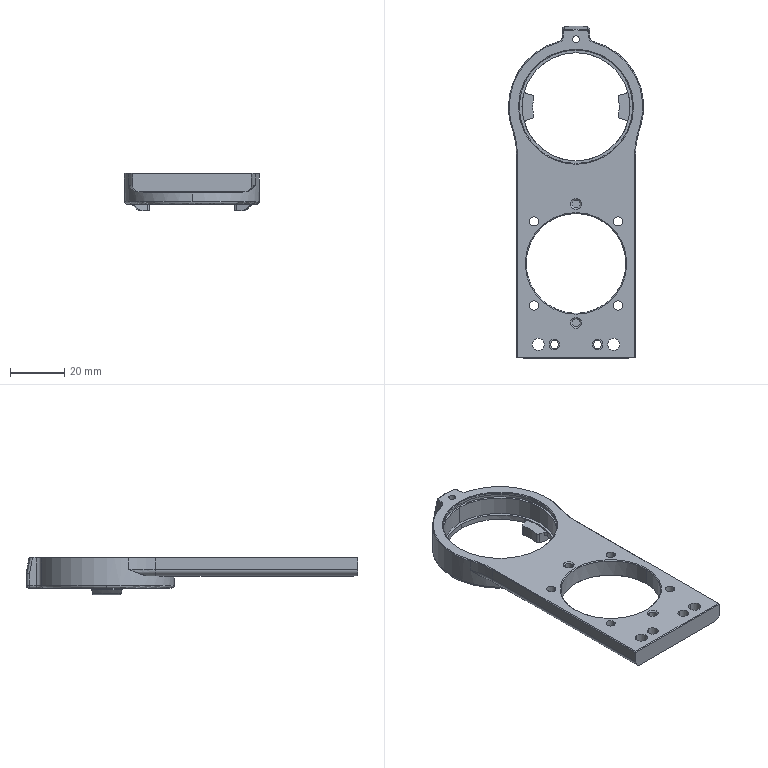NC program | NX | posted with a generic post | part box 50 x 122.9 x 14 mm
Lines 869 to 1773 of 10876:
(FLOOR_WALL_1_COPY_1 , TOOL : D4)
N1712 T11 M6
N1714 G54
N1716 G17 G0 G90 X62.415 Y-8.2 S9500 M3
N1718 G43 Z30. H11
N1720 Z-0.5
N1722 G94 G1 X62.153 Y-7.279 Z-0.55 F1000.
N1724 X61.62 Y-4.45 Z-0.701
N1726 X61.486 Y-3.078 Z-0.773
N1728 X61.34 Y-4.335 Z-0.84
N1730 X60.809 Y-6.819 Z-0.973
N1732 X60.044 Y-9.241 Z-1.106
N1734 X59.55 Y-10.406 Z-1.172
N1736 X59.81 Y-10.859 Z-1.2
N1738 X60.022 Y-11.336 Z-1.227
N1740 X63.435 Z-1.406
N1742 X62.941 Y-10.049 Z-1.478
N1744 X62.153 Y-7.279 Z-1.629
N1746 X61.62 Y-4.45 Z-1.78
N1748 X61.486 Y-3.078 Z-1.852
N1750 X61.34 Y-4.335 Z-1.918
N1752 X60.809 Y-6.819 Z-2.051
N1754 X60.044 Y-9.241 Z-2.185
N1756 X59.55 Y-10.406 Z-2.251
N1758 X59.81 Y-10.859 Z-2.278
N1760 X60.022 Y-11.336 Z-2.306
N1762 X61.728 Z-2.395
N1764 X63.435 F2000.
N1766 G2 X61.486 Y-3.078 R31.664
N1768 X59.55 Y-10.406 R26.664
N1770 X60.022 Y-11.336 R10.364
N1772 G1 X61.728
N1774 Y-13.336
N1776 X66.503
N1778 G2 X63.476 Y2.884 R29.664
N1780 G1 X61.486 Y3.078
N1782 G2 X63.435 Y11.336 R31.664
N1784 G1 X60.022
N1786 G2 X59.55 Y10.406 R10.364
N1788 X61.486 Y3.078 R26.664
N1790 G1 X63.476 Y2.884
N1792 G2 X66.503 Y13.336 R29.664
N1794 G1 X58.62
N1796 G2 X57.279 Y10.581 R8.364
N1798 X57.279 Y-10.581 R24.664
N1800 X58.62 Y-13.336 R8.364
N1802 G1 X61.728
N1804 Y-15.336
N1806 X69.976
N1808 G2 X69.976 Y15.336 R27.664
N1810 G1 X56.917
N1812 G2 X54.879 Y10.885 R6.364
N1814 X54.879 Y-10.885 R22.664
N1816 X56.917 Y-15.336 R6.364
N1818 G1 X61.728
N1820 Z-0.895
N1822 G0 X62.415 Y-8.2
N1824 G1 X62.153 Y-7.279 Z-0.945 F1000.
N1826 X61.62 Y-4.45 Z-1.096
N1828 X61.486 Y-3.078 Z-1.168
N1830 X61.34 Y-4.335 Z-1.235
N1832 X60.809 Y-6.819 Z-1.368
N1834 X60.044 Y-9.241 Z-1.501
N1836 X59.55 Y-10.406 Z-1.567
N1838 X59.81 Y-10.859 Z-1.595
N1840 X60.022 Y-11.336 Z-1.622
N1842 X63.435 Z-1.801
N1844 X62.941 Y-10.049 Z-1.873
N1846 X62.153 Y-7.279 Z-2.024
N1848 X61.62 Y-4.45 Z-2.175
N1850 X61.486 Y-3.078 Z-2.247
N1852 X61.34 Y-4.335 Z-2.313
N1854 X60.809 Y-6.819 Z-2.446
N1856 X60.044 Y-9.241 Z-2.58
N1858 X59.55 Y-10.406 Z-2.646
N1860 X59.81 Y-10.859 Z-2.673
N1862 X60.022 Y-11.336 Z-2.701
N1864 X61.728 Z-2.79
N1866 X63.435 F2000.
N1868 G2 X61.486 Y-3.078 R31.664
N1870 X59.55 Y-10.406 R26.664
N1872 X60.022 Y-11.336 R10.364
N1874 G1 X61.728
N1876 Y-13.336
N1878 X66.503
N1880 G2 X63.476 Y2.884 R29.664
N1882 G1 X61.486 Y3.078
N1884 G2 X63.435 Y11.336 R31.664
N1886 G1 X60.022
N1888 G2 X59.55 Y10.406 R10.364
N1890 X61.486 Y3.078 R26.664
N1892 G1 X63.476 Y2.884
N1894 G2 X66.503 Y13.336 R29.664
N1896 G1 X58.62
N1898 G2 X57.279 Y10.581 R8.364
N1900 X57.279 Y-10.581 R24.664
N1902 X58.62 Y-13.336 R8.364
N1904 G1 X61.728
N1906 Y-15.336
N1908 X69.976
N1910 G2 X69.976 Y15.336 R27.664
N1912 G1 X56.917
N1914 G2 X54.879 Y10.885 R6.364
N1916 X54.879 Y-10.885 R22.664
N1918 X56.917 Y-15.336 R6.364
N1920 G1 X61.728
N1922 Z-1.29
N1924 G0 X62.415 Y-8.2
N1926 G1 X62.153 Y-7.279 Z-1.34 F1000.
N1928 X61.62 Y-4.45 Z-1.491
N1930 X61.486 Y-3.078 Z-1.563
N1932 X61.34 Y-4.335 Z-1.63
N1934 X60.809 Y-6.819 Z-1.763
N1936 X60.044 Y-9.241 Z-1.896
N1938 X59.55 Y-10.406 Z-1.962
N1940 X59.81 Y-10.859 Z-1.99
N1942 X60.022 Y-11.336 Z-2.017
N1944 X63.435 Z-2.196
N1946 X62.941 Y-10.049 Z-2.268
N1948 X62.153 Y-7.279 Z-2.419
N1950 X61.62 Y-4.45 Z-2.57
N1952 X61.486 Y-3.078 Z-2.642
N1954 X61.34 Y-4.335 Z-2.708
N1956 X60.809 Y-6.819 Z-2.841
N1958 X60.044 Y-9.241 Z-2.975
N1960 X59.55 Y-10.406 Z-3.041
N1962 X59.81 Y-10.859 Z-3.068
N1964 X60.022 Y-11.336 Z-3.096
N1966 X61.728 Z-3.185
N1968 X63.435 F2000.
N1970 G2 X61.486 Y-3.078 R31.664
N1972 X59.55 Y-10.406 R26.664
N1974 X60.022 Y-11.336 R10.364
N1976 G1 X61.728
N1978 Y-13.336
N1980 X66.503
N1982 G2 X63.476 Y2.884 R29.664
N1984 G1 X61.486 Y3.078
N1986 G2 X63.435 Y11.336 R31.664
N1988 G1 X60.022
N1990 G2 X59.55 Y10.406 R10.364
N1992 X61.486 Y3.078 R26.664
N1994 G1 X63.476 Y2.884
N1996 G2 X66.503 Y13.336 R29.664
N1998 G1 X58.62
N2000 G2 X57.279 Y10.581 R8.364
N2002 X57.279 Y-10.581 R24.664
N2004 X58.62 Y-13.336 R8.364
N2006 G1 X61.728
N2008 Y-15.336
N2010 X69.976
N2012 G2 X69.976 Y15.336 R27.664
N2014 G1 X56.917
N2016 G2 X54.879 Y10.885 R6.364
N2018 X54.879 Y-10.885 R22.664
N2020 X56.917 Y-15.336 R6.364
N2022 G1 X61.728
N2024 Z-1.685
N2026 G0 X62.415 Y-8.2
N2028 G1 X62.153 Y-7.279 Z-1.735 F1000.
N2030 X61.62 Y-4.45 Z-1.886
N2032 X61.486 Y-3.078 Z-1.958
N2034 X61.34 Y-4.335 Z-2.025
N2036 X60.809 Y-6.819 Z-2.158
N2038 X60.044 Y-9.241 Z-2.291
N2040 X59.55 Y-10.406 Z-2.357
N2042 X59.81 Y-10.859 Z-2.385
N2044 X60.022 Y-11.336 Z-2.412
N2046 X63.435 Z-2.591
N2048 X62.941 Y-10.049 Z-2.663
N2050 X62.153 Y-7.279 Z-2.814
N2052 X61.62 Y-4.45 Z-2.965
N2054 X61.486 Y-3.078 Z-3.037
N2056 X61.34 Y-4.335 Z-3.103
N2058 X60.809 Y-6.819 Z-3.236
N2060 X60.044 Y-9.241 Z-3.37
N2062 X59.55 Y-10.406 Z-3.436
N2064 X59.81 Y-10.859 Z-3.463
N2066 X60.022 Y-11.336 Z-3.491
N2068 X61.728 Z-3.58
N2070 X63.435 F2000.
N2072 G2 X61.486 Y-3.078 R31.664
N2074 X59.55 Y-10.406 R26.664
N2076 X60.022 Y-11.336 R10.364
N2078 G1 X61.728
N2080 Y-13.336
N2082 X66.503
N2084 G2 X63.476 Y2.884 R29.664
N2086 G1 X61.486 Y3.078
N2088 G2 X63.435 Y11.336 R31.664
N2090 G1 X60.022
N2092 G2 X59.55 Y10.406 R10.364
N2094 X61.486 Y3.078 R26.664
N2096 G1 X63.476 Y2.884
N2098 G2 X66.503 Y13.336 R29.664
N2100 G1 X58.62
N2102 G2 X57.279 Y10.581 R8.364
N2104 X57.279 Y-10.581 R24.664
N2106 X58.62 Y-13.336 R8.364
N2108 G1 X61.728
N2110 Y-15.336
N2112 X69.976
N2114 G2 X69.976 Y15.336 R27.664
N2116 G1 X56.917
N2118 G2 X54.879 Y10.885 R6.364
N2120 X54.879 Y-10.885 R22.664
N2122 X56.917 Y-15.336 R6.364
N2124 G1 X61.728
N2126 Z-2.08
N2128 G0 X62.415 Y-8.2
N2130 G1 X62.153 Y-7.279 Z-2.13 F1000.
N2132 X61.62 Y-4.45 Z-2.281
N2134 X61.486 Y-3.078 Z-2.353
N2136 X61.34 Y-4.335 Z-2.42
N2138 X60.809 Y-6.819 Z-2.553
N2140 X60.044 Y-9.241 Z-2.686
N2142 X59.55 Y-10.406 Z-2.752
N2144 X59.81 Y-10.859 Z-2.78
N2146 X60.022 Y-11.336 Z-2.807
N2148 X63.435 Z-2.986
N2150 X62.941 Y-10.049 Z-3.058
N2152 X62.153 Y-7.279 Z-3.209
N2154 X61.62 Y-4.45 Z-3.36
N2156 X61.486 Y-3.078 Z-3.432
N2158 X61.34 Y-4.335 Z-3.498
N2160 X60.809 Y-6.819 Z-3.631
N2162 X60.044 Y-9.241 Z-3.765
N2164 X59.55 Y-10.406 Z-3.831
N2166 X59.81 Y-10.859 Z-3.858
N2168 X60.022 Y-11.336 Z-3.886
N2170 X61.728 Z-3.975
N2172 X63.435 F2000.
N2174 G2 X61.486 Y-3.078 R31.664
N2176 X59.55 Y-10.406 R26.664
N2178 X60.022 Y-11.336 R10.364
N2180 G1 X61.728
N2182 Y-13.336
N2184 X66.503
N2186 G2 X63.476 Y2.884 R29.664
N2188 G1 X61.486 Y3.078
N2190 G2 X63.435 Y11.336 R31.664
N2192 G1 X60.022
N2194 G2 X59.55 Y10.406 R10.364
N2196 X61.486 Y3.078 R26.664
N2198 G1 X63.476 Y2.884
N2200 G2 X66.503 Y13.336 R29.664
N2202 G1 X58.62
N2204 G2 X57.279 Y10.581 R8.364
N2206 X57.279 Y-10.581 R24.664
N2208 X58.62 Y-13.336 R8.364
N2210 G1 X61.728
N2212 Y-15.336
N2214 X69.976
N2216 G2 X69.976 Y15.336 R27.664
N2218 G1 X56.917
N2220 G2 X54.879 Y10.885 R6.364
N2222 X54.879 Y-10.885 R22.664
N2224 X56.917 Y-15.336 R6.364
N2226 G1 X61.728
N2228 Z-2.475
N2230 G0 X62.415 Y-8.2
N2232 G1 X62.153 Y-7.279 Z-2.525 F1000.
N2234 X61.62 Y-4.45 Z-2.676
N2236 X61.486 Y-3.078 Z-2.748
N2238 X61.34 Y-4.335 Z-2.815
N2240 X60.809 Y-6.819 Z-2.948
N2242 X60.044 Y-9.241 Z-3.081
N2244 X59.55 Y-10.406 Z-3.147
N2246 X59.81 Y-10.859 Z-3.175
N2248 X60.022 Y-11.336 Z-3.202
N2250 X63.435 Z-3.381
N2252 X62.941 Y-10.049 Z-3.453
N2254 X62.153 Y-7.279 Z-3.604
N2256 X61.62 Y-4.45 Z-3.755
N2258 X61.486 Y-3.078 Z-3.827
N2260 X61.34 Y-4.335 Z-3.893
N2262 X60.809 Y-6.819 Z-4.026
N2264 X60.044 Y-9.241 Z-4.16
N2266 X59.55 Y-10.406 Z-4.226
N2268 X59.81 Y-10.859 Z-4.253
N2270 X60.022 Y-11.336 Z-4.281
N2272 X61.728 Z-4.37
N2274 X63.435 F2000.
N2276 G2 X61.486 Y-3.078 R31.664
N2278 X59.55 Y-10.406 R26.664
N2280 X60.022 Y-11.336 R10.364
N2282 G1 X61.728
N2284 Y-13.336
N2286 X66.503
N2288 G2 X63.476 Y2.884 R29.664
N2290 G1 X61.486 Y3.078
N2292 G2 X63.435 Y11.336 R31.664
N2294 G1 X60.022
N2296 G2 X59.55 Y10.406 R10.364
N2298 X61.486 Y3.078 R26.664
N2300 G1 X63.476 Y2.884
N2302 G2 X66.503 Y13.336 R29.664
N2304 G1 X58.62
N2306 G2 X57.279 Y10.581 R8.364
N2308 X57.279 Y-10.581 R24.664
N2310 X58.62 Y-13.336 R8.364
N2312 G1 X61.728
N2314 Y-15.336
N2316 X69.976
N2318 G2 X69.976 Y15.336 R27.664
N2320 G1 X56.917
N2322 G2 X54.879 Y10.885 R6.364
N2324 X54.879 Y-10.885 R22.664
N2326 X56.917 Y-15.336 R6.364
N2328 G1 X61.728
N2330 Z-2.87
N2332 G0 X62.415 Y-8.2
N2334 G1 X62.153 Y-7.279 Z-2.92 F1000.
N2336 X61.62 Y-4.45 Z-3.071
N2338 X61.486 Y-3.078 Z-3.143
N2340 X61.34 Y-4.335 Z-3.21
N2342 X60.809 Y-6.819 Z-3.343
N2344 X60.044 Y-9.241 Z-3.476
N2346 X59.55 Y-10.406 Z-3.542
N2348 X59.81 Y-10.859 Z-3.57
N2350 X60.022 Y-11.336 Z-3.597
N2352 X63.435 Z-3.776
N2354 X62.941 Y-10.049 Z-3.848
N2356 X62.153 Y-7.279 Z-3.999
N2358 X61.62 Y-4.45 Z-4.15
N2360 X61.486 Y-3.078 Z-4.222
N2362 X61.34 Y-4.335 Z-4.288
N2364 X60.809 Y-6.819 Z-4.421
N2366 X60.044 Y-9.241 Z-4.555
N2368 X59.55 Y-10.406 Z-4.621
N2370 X59.81 Y-10.859 Z-4.648
N2372 X60.022 Y-11.336 Z-4.676
N2374 X61.728 Z-4.765
N2376 X63.435 F2000.
N2378 G2 X61.486 Y-3.078 R31.664
N2380 X59.55 Y-10.406 R26.664
N2382 X60.022 Y-11.336 R10.364
N2384 G1 X61.728
N2386 Y-13.336
N2388 X66.503
N2390 G2 X63.476 Y2.884 R29.664
N2392 G1 X61.486 Y3.078
N2394 G2 X63.435 Y11.336 R31.664
N2396 G1 X60.022
N2398 G2 X59.55 Y10.406 R10.364
N2400 X61.486 Y3.078 R26.664
N2402 G1 X63.476 Y2.884
N2404 G2 X66.503 Y13.336 R29.664
N2406 G1 X58.62
N2408 G2 X57.279 Y10.581 R8.364
N2410 X57.279 Y-10.581 R24.664
N2412 X58.62 Y-13.336 R8.364
N2414 G1 X61.728
N2416 Y-15.336
N2418 X69.976
N2420 G2 X69.976 Y15.336 R27.664
N2422 G1 X56.917
N2424 G2 X54.879 Y10.885 R6.364
N2426 X54.879 Y-10.885 R22.664
N2428 X56.917 Y-15.336 R6.364
N2430 G1 X61.728
N2432 Z-3.265
N2434 G0 X62.415 Y-8.2
N2436 G1 X62.153 Y-7.279 Z-3.315 F1000.
N2438 X61.62 Y-4.45 Z-3.466
N2440 X61.486 Y-3.078 Z-3.538
N2442 X61.34 Y-4.335 Z-3.605
N2444 X60.809 Y-6.819 Z-3.738
N2446 X60.044 Y-9.241 Z-3.871
N2448 X59.55 Y-10.406 Z-3.937
N2450 X59.81 Y-10.859 Z-3.965
N2452 X60.022 Y-11.336 Z-3.992
N2454 X63.435 Z-4.171
N2456 X62.941 Y-10.049 Z-4.243
N2458 X62.153 Y-7.279 Z-4.394
N2460 X61.62 Y-4.45 Z-4.545
N2462 X61.486 Y-3.078 Z-4.617
N2464 X61.34 Y-4.335 Z-4.683
N2466 X60.809 Y-6.819 Z-4.816
N2468 X60.044 Y-9.241 Z-4.95
N2470 X59.55 Y-10.406 Z-5.016
N2472 X59.81 Y-10.859 Z-5.043
N2474 X60.022 Y-11.336 Z-5.071
N2476 X61.728 Z-5.16
N2478 X63.435 F2000.
N2480 G2 X61.486 Y-3.078 R31.664
N2482 X59.55 Y-10.406 R26.664
N2484 X60.022 Y-11.336 R10.364
N2486 G1 X61.728
N2488 Y-13.336
N2490 X66.503
N2492 G2 X63.476 Y2.884 R29.664
N2494 G1 X61.486 Y3.078
N2496 G2 X63.435 Y11.336 R31.664
N2498 G1 X60.022
N2500 G2 X59.55 Y10.406 R10.364
N2502 X61.486 Y3.078 R26.664
N2504 G1 X63.476 Y2.884
N2506 G2 X66.503 Y13.336 R29.664
N2508 G1 X58.62
N2510 G2 X57.279 Y10.581 R8.364
N2512 X57.279 Y-10.581 R24.664
N2514 X58.62 Y-13.336 R8.364
N2516 G1 X61.728
N2518 Y-15.336
N2520 X69.976
N2522 G2 X69.976 Y15.336 R27.664
N2524 G1 X56.917
N2526 G2 X54.879 Y10.885 R6.364
N2528 X54.879 Y-10.885 R22.664
N2530 X56.917 Y-15.336 R6.364
N2532 G1 X61.728
N2534 Z-3.66
N2536 G0 X62.415 Y-8.2
N2538 G1 X62.153 Y-7.279 Z-3.71 F1000.
N2540 X61.62 Y-4.45 Z-3.861
N2542 X61.486 Y-3.078 Z-3.933
N2544 X61.34 Y-4.335 Z-4.
N2546 X60.809 Y-6.819 Z-4.133
N2548 X60.044 Y-9.241 Z-4.266
N2550 X59.55 Y-10.406 Z-4.332
N2552 X59.81 Y-10.859 Z-4.36
N2554 X60.022 Y-11.336 Z-4.387
N2556 X63.435 Z-4.566
N2558 X62.941 Y-10.049 Z-4.638
N2560 X62.153 Y-7.279 Z-4.789
N2562 X61.62 Y-4.45 Z-4.94
N2564 X61.486 Y-3.078 Z-5.012
N2566 X61.34 Y-4.335 Z-5.078
N2568 X60.809 Y-6.819 Z-5.211
N2570 X60.044 Y-9.241 Z-5.345
N2572 X59.55 Y-10.406 Z-5.411
N2574 X59.81 Y-10.859 Z-5.438
N2576 X60.022 Y-11.336 Z-5.466
N2578 X61.728 Z-5.555
N2580 X63.435 F2000.
N2582 G2 X61.486 Y-3.078 R31.664
N2584 X59.55 Y-10.406 R26.664
N2586 X60.022 Y-11.336 R10.364
N2588 G1 X61.728
N2590 Y-13.336
N2592 X66.503
N2594 G2 X63.476 Y2.884 R29.664
N2596 G1 X61.486 Y3.078
N2598 G2 X63.435 Y11.336 R31.664
N2600 G1 X60.022
N2602 G2 X59.55 Y10.406 R10.364
N2604 X61.486 Y3.078 R26.664
N2606 G1 X63.476 Y2.884
N2608 G2 X66.503 Y13.336 R29.664
N2610 G1 X58.62
N2612 G2 X57.279 Y10.581 R8.364
N2614 X57.279 Y-10.581 R24.664
N2616 X58.62 Y-13.336 R8.364
N2618 G1 X61.728
N2620 Y-15.336
N2622 X69.976
N2624 G2 X69.976 Y15.336 R27.664
N2626 G1 X56.917
N2628 G2 X54.879 Y10.885 R6.364
N2630 X54.879 Y-10.885 R22.664
N2632 X56.917 Y-15.336 R6.364
N2634 G1 X61.728
N2636 Z-4.055
N2638 G0 X62.415 Y-8.2
N2640 G1 X62.153 Y-7.279 Z-4.105 F1000.
N2642 X61.62 Y-4.45 Z-4.256
N2644 X61.486 Y-3.078 Z-4.328
N2646 X61.34 Y-4.335 Z-4.395
N2648 X60.809 Y-6.819 Z-4.528
N2650 X60.044 Y-9.241 Z-4.661
N2652 X59.55 Y-10.406 Z-4.727
N2654 X59.81 Y-10.859 Z-4.755
N2656 X60.022 Y-11.336 Z-4.782
N2658 X63.435 Z-4.961
N2660 X62.941 Y-10.049 Z-5.033
N2662 X62.153 Y-7.279 Z-5.184
N2664 X61.62 Y-4.45 Z-5.335
N2666 X61.486 Y-3.078 Z-5.407
N2668 X61.34 Y-4.335 Z-5.473
N2670 X60.809 Y-6.819 Z-5.606
N2672 X60.044 Y-9.241 Z-5.74
N2674 X59.55 Y-10.406 Z-5.806
N2676 X59.81 Y-10.859 Z-5.833
N2678 X60.022 Y-11.336 Z-5.861
N2680 X61.728 Z-5.95
N2682 X63.435 F2000.
N2684 G2 X61.486 Y-3.078 R31.664
N2686 X59.55 Y-10.406 R26.664
N2688 X60.022 Y-11.336 R10.364
N2690 G1 X61.728
N2692 Y-13.336
N2694 X66.503
N2696 G2 X63.476 Y2.884 R29.664
N2698 G1 X61.486 Y3.078
N2700 G2 X63.435 Y11.336 R31.664
N2702 G1 X60.022
N2704 G2 X59.55 Y10.406 R10.364
N2706 X61.486 Y3.078 R26.664
N2708 G1 X63.476 Y2.884
N2710 G2 X66.503 Y13.336 R29.664
N2712 G1 X58.62
N2714 G2 X57.279 Y10.581 R8.364
N2716 X57.279 Y-10.581 R24.664
N2718 X58.62 Y-13.336 R8.364
N2720 G1 X61.728
N2722 Y-15.336
N2724 X69.976
N2726 G2 X69.976 Y15.336 R27.664
N2728 G1 X56.917
N2730 G2 X54.879 Y10.885 R6.364
N2732 X54.879 Y-10.885 R22.664
N2734 X56.917 Y-15.336 R6.364
N2736 G1 X61.728
N2738 Z-4.45
N2740 G0 X62.415 Y-8.2
N2742 G1 X62.153 Y-7.279 Z-4.5 F1000.
N2744 X61.62 Y-4.45 Z-4.651
N2746 X61.486 Y-3.078 Z-4.723
N2748 X61.34 Y-4.335 Z-4.79
N2750 X60.809 Y-6.819 Z-4.923
N2752 X60.044 Y-9.241 Z-5.056
N2754 X59.55 Y-10.406 Z-5.122
N2756 X59.81 Y-10.859 Z-5.15
N2758 X60.022 Y-11.336 Z-5.177
N2760 X63.435 Z-5.356
N2762 X62.941 Y-10.049 Z-5.428
N2764 X62.153 Y-7.279 Z-5.579
N2766 X61.62 Y-4.45 Z-5.73
N2768 X61.486 Y-3.078 Z-5.802
N2770 X61.34 Y-4.335 Z-5.868
N2772 X60.809 Y-6.819 Z-6.001
N2774 X60.044 Y-9.241 Z-6.135
N2776 X59.55 Y-10.406 Z-6.201
N2778 X59.81 Y-10.859 Z-6.228
N2780 X60.022 Y-11.336 Z-6.256
N2782 X61.728 Z-6.345
N2784 X63.435 F2000.
N2786 G2 X61.486 Y-3.078 R31.664
N2788 X59.55 Y-10.406 R26.664
N2790 X60.022 Y-11.336 R10.364
N2792 G1 X61.728
N2794 Y-13.336
N2796 X66.503
N2798 G2 X63.476 Y2.884 R29.664
N2800 G1 X61.486 Y3.078
N2802 G2 X63.435 Y11.336 R31.664
N2804 G1 X60.022
N2806 G2 X59.55 Y10.406 R10.364
N2808 X61.486 Y3.078 R26.664
N2810 G1 X63.476 Y2.884
N2812 G2 X66.503 Y13.336 R29.664
N2814 G1 X58.62
N2816 G2 X57.279 Y10.581 R8.364
N2818 X57.279 Y-10.581 R24.664
N2820 X58.62 Y-13.336 R8.364
N2822 G1 X61.728
N2824 Y-15.336
N2826 X69.976
N2828 G2 X69.976 Y15.336 R27.664
N2830 G1 X56.917
N2832 G2 X54.879 Y10.885 R6.364
N2834 X54.879 Y-10.885 R22.664
N2836 X56.917 Y-15.336 R6.364
N2838 G1 X61.728
N2840 Z-4.845
N2842 G0 X62.415 Y-8.2
N2844 G1 X62.153 Y-7.279 Z-4.895 F1000.
N2846 X61.62 Y-4.45 Z-5.046
N2848 X61.486 Y-3.078 Z-5.118
N2850 X61.34 Y-4.335 Z-5.185
N2852 X60.809 Y-6.819 Z-5.318
N2854 X60.044 Y-9.241 Z-5.451
N2856 X59.55 Y-10.406 Z-5.517
N2858 X59.81 Y-10.859 Z-5.545
N2860 X60.022 Y-11.336 Z-5.572
N2862 X63.435 Z-5.751
N2864 X62.941 Y-10.049 Z-5.823
N2866 X62.153 Y-7.279 Z-5.974
N2868 X61.62 Y-4.45 Z-6.125
N2870 X61.486 Y-3.078 Z-6.197
N2872 X61.34 Y-4.335 Z-6.263
N2874 X60.809 Y-6.819 Z-6.396
N2876 X60.044 Y-9.241 Z-6.53
N2878 X59.55 Y-10.406 Z-6.596
N2880 X59.81 Y-10.859 Z-6.623
N2882 X60.022 Y-11.336 Z-6.651
N2884 X61.728 Z-6.74
N2886 X63.435 F2000.
N2888 G2 X61.486 Y-3.078 R31.664
N2890 X59.55 Y-10.406 R26.664
N2892 X60.022 Y-11.336 R10.364
N2894 G1 X61.728
N2896 Y-13.336
N2898 X66.503
N2900 G2 X63.476 Y2.884 R29.664
N2902 G1 X61.486 Y3.078
N2904 G2 X63.435 Y11.336 R31.664
N2906 G1 X60.022
N2908 G2 X59.55 Y10.406 R10.364
N2910 X61.486 Y3.078 R26.664
N2912 G1 X63.476 Y2.884
N2914 G2 X66.503 Y13.336 R29.664
N2916 G1 X58.62
N2918 G2 X57.279 Y10.581 R8.364
N2920 X57.279 Y-10.581 R24.664
N2922 X58.62 Y-13.336 R8.364
N2924 G1 X61.728
N2926 Y-15.336
N2928 X69.976
N2930 G2 X69.976 Y15.336 R27.664
N2932 G1 X56.917
N2934 G2 X54.879 Y10.885 R6.364
N2936 X54.879 Y-10.885 R22.664
N2938 X56.917 Y-15.336 R6.364
N2940 G1 X61.728
N2942 Z-5.24
N2944 G0 X62.415 Y-8.2
N2946 G1 X62.153 Y-7.279 Z-5.29 F1000.
N2948 X61.62 Y-4.45 Z-5.441
N2950 X61.486 Y-3.078 Z-5.513
N2952 X61.34 Y-4.335 Z-5.58
N2954 X60.809 Y-6.819 Z-5.713
N2956 X60.044 Y-9.241 Z-5.846
N2958 X59.55 Y-10.406 Z-5.912
N2960 X59.81 Y-10.859 Z-5.94
N2962 X60.022 Y-11.336 Z-5.967
N2964 X63.435 Z-6.146
N2966 X62.941 Y-10.049 Z-6.218
N2968 X62.153 Y-7.279 Z-6.369
N2970 X61.62 Y-4.45 Z-6.52
N2972 X61.486 Y-3.078 Z-6.592
N2974 X61.34 Y-4.335 Z-6.658
N2976 X60.809 Y-6.819 Z-6.791
N2978 X60.044 Y-9.241 Z-6.925
N2980 X59.55 Y-10.406 Z-6.991
N2982 X59.81 Y-10.859 Z-7.018
N2984 X60.022 Y-11.336 Z-7.046
N2986 X61.728 Z-7.135
N2988 X63.435 F2000.
N2990 G2 X61.486 Y-3.078 R31.664
N2992 X59.55 Y-10.406 R26.664
N2994 X60.022 Y-11.336 R10.364
N2996 G1 X61.728
N2998 Y-13.336
N3000 X66.503
N3002 G2 X63.476 Y2.884 R29.664
N3004 G1 X61.486 Y3.078
N3006 G2 X63.435 Y11.336 R31.664
N3008 G1 X60.022
N3010 G2 X59.55 Y10.406 R10.364
N3012 X61.486 Y3.078 R26.664
N3014 G1 X63.476 Y2.884
N3016 G2 X66.503 Y13.336 R29.664
N3018 G1 X58.62
N3020 G2 X57.279 Y10.581 R8.364
N3022 X57.279 Y-10.581 R24.664
N3024 X58.62 Y-13.336 R8.364
N3026 G1 X61.728
N3028 Y-15.336
N3030 X69.976
N3032 G2 X69.976 Y15.336 R27.664
N3034 G1 X56.917
N3036 G2 X54.879 Y10.885 R6.364
N3038 X54.879 Y-10.885 R22.664
N3040 X56.917 Y-15.336 R6.364
N3042 G1 X61.728
N3044 Z-5.635
N3046 G0 X62.415 Y-8.2
N3048 G1 X62.153 Y-7.279 Z-5.685 F1000.
N3050 X61.62 Y-4.45 Z-5.836
N3052 X61.486 Y-3.078 Z-5.908
N3054 X61.34 Y-4.335 Z-5.975
N3056 X60.809 Y-6.819 Z-6.108
N3058 X60.044 Y-9.241 Z-6.241
N3060 X59.55 Y-10.406 Z-6.307
N3062 X59.81 Y-10.859 Z-6.335
N3064 X60.022 Y-11.336 Z-6.362
N3066 X63.435 Z-6.541
N3068 X62.941 Y-10.049 Z-6.613
N3070 X62.153 Y-7.279 Z-6.764
N3072 X61.62 Y-4.45 Z-6.915
N3074 X61.486 Y-3.078 Z-6.987
N3076 X61.34 Y-4.335 Z-7.053
N3078 X60.809 Y-6.819 Z-7.186
N3080 X60.044 Y-9.241 Z-7.32
N3082 X59.55 Y-10.406 Z-7.386
N3084 X59.81 Y-10.859 Z-7.413
N3086 X60.022 Y-11.336 Z-7.441
N3088 X61.728 Z-7.53
N3090 X63.435 F2000.
N3092 G2 X61.486 Y-3.078 R31.664
N3094 X59.55 Y-10.406 R26.664
N3096 X60.022 Y-11.336 R10.364
N3098 G1 X61.728
N3100 Y-13.336
N3102 X66.503
N3104 G2 X63.476 Y2.884 R29.664
N3106 G1 X61.486 Y3.078
N3108 G2 X63.435 Y11.336 R31.664
N3110 G1 X60.022
N3112 G2 X59.55 Y10.406 R10.364
N3114 X61.486 Y3.078 R26.664
N3116 G1 X63.476 Y2.884
N3118 G2 X66.503 Y13.336 R29.664
N3120 G1 X58.62
N3122 G2 X57.279 Y10.581 R8.364
N3124 X57.279 Y-10.581 R24.664
N3126 X58.62 Y-13.336 R8.364
N3128 G1 X61.728
N3130 Y-15.336
N3132 X69.976
N3134 G2 X69.976 Y15.336 R27.664
N3136 G1 X56.917
N3138 G2 X54.879 Y10.885 R6.364
N3140 X54.879 Y-10.885 R22.664
N3142 X56.917 Y-15.336 R6.364
N3144 G1 X61.728
N3146 Z-6.03
N3148 G0 X62.415 Y-8.2
N3150 G1 X62.153 Y-7.279 Z-6.08 F1000.
N3152 X61.62 Y-4.45 Z-6.231
N3154 X61.486 Y-3.078 Z-6.303
N3156 X61.34 Y-4.335 Z-6.37
N3158 X60.809 Y-6.819 Z-6.503
N3160 X60.044 Y-9.241 Z-6.636
N3162 X59.55 Y-10.406 Z-6.702
N3164 X59.81 Y-10.859 Z-6.73
N3166 X60.022 Y-11.336 Z-6.757
N3168 X63.435 Z-6.936
N3170 X62.941 Y-10.049 Z-7.008
N3172 X62.153 Y-7.279 Z-7.159
N3174 X61.62 Y-4.45 Z-7.31
N3176 X61.486 Y-3.078 Z-7.382
N3178 X61.34 Y-4.335 Z-7.448
N3180 X60.809 Y-6.819 Z-7.581
N3182 X60.044 Y-9.241 Z-7.715
N3184 X59.55 Y-10.406 Z-7.781
N3186 X59.81 Y-10.859 Z-7.808
N3188 X60.022 Y-11.336 Z-7.836
N3190 X61.728 Z-7.925
N3192 X63.435 F2000.
N3194 G2 X61.486 Y-3.078 R31.664
N3196 X59.55 Y-10.406 R26.664
N3198 X60.022 Y-11.336 R10.364
N3200 G1 X61.728
N3202 Y-13.336
N3204 X66.503
N3206 G2 X63.476 Y2.884 R29.664
N3208 G1 X61.486 Y3.078
N3210 G2 X63.435 Y11.336 R31.664
N3212 G1 X60.022
N3214 G2 X59.55 Y10.406 R10.364
N3216 X61.486 Y3.078 R26.664
N3218 G1 X63.476 Y2.884
N3220 G2 X66.503 Y13.336 R29.664
N3222 G1 X58.62
N3224 G2 X57.279 Y10.581 R8.364
N3226 X57.279 Y-10.581 R24.664
N3228 X58.62 Y-13.336 R8.364
N3230 G1 X61.728
N3232 Y-15.336
N3234 X69.976
N3236 G2 X69.976 Y15.336 R27.664
N3238 G1 X56.917
N3240 G2 X54.879 Y10.885 R6.364
N3242 X54.879 Y-10.885 R22.664
N3244 X56.917 Y-15.336 R6.364
N3246 G1 X61.728
N3248 Z-6.425
N3250 G0 X62.415 Y-8.2
N3252 G1 X62.153 Y-7.279 Z-6.475 F1000.
N3254 X61.62 Y-4.45 Z-6.626
N3256 X61.486 Y-3.078 Z-6.698
N3258 X61.34 Y-4.335 Z-6.765
N3260 X60.809 Y-6.819 Z-6.898
N3262 X60.044 Y-9.241 Z-7.031
N3264 X59.55 Y-10.406 Z-7.097
N3266 X59.81 Y-10.859 Z-7.125
N3268 X60.022 Y-11.336 Z-7.152
N3270 X63.435 Z-7.331
N3272 X62.941 Y-10.049 Z-7.403
N3274 X62.153 Y-7.279 Z-7.554
N3276 X61.62 Y-4.45 Z-7.705
N3278 X61.486 Y-3.078 Z-7.777
N3280 X61.34 Y-4.335 Z-7.843
N3282 X60.809 Y-6.819 Z-7.976
N3284 X60.044 Y-9.241 Z-8.11
N3286 X59.55 Y-10.406 Z-8.176
N3288 X59.81 Y-10.859 Z-8.203
N3290 X60.022 Y-11.336 Z-8.231
N3292 X61.728 Z-8.32
N3294 X63.435 F2000.
N3296 G2 X61.486 Y-3.078 R31.664
N3298 X59.55 Y-10.406 R26.664
N3300 X60.022 Y-11.336 R10.364
N3302 G1 X61.728
N3304 Y-13.336
N3306 X66.503
N3308 G2 X63.476 Y2.884 R29.664
N3310 G1 X61.486 Y3.078
N3312 G2 X63.435 Y11.336 R31.664
N3314 G1 X60.022
N3316 G2 X59.55 Y10.406 R10.364
N3318 X61.486 Y3.078 R26.664
N3320 G1 X63.476 Y2.884
N3322 G2 X66.503 Y13.336 R29.664
N3324 G1 X58.62
N3326 G2 X57.279 Y10.581 R8.364
N3328 X57.279 Y-10.581 R24.664
N3330 X58.62 Y-13.336 R8.364
N3332 G1 X61.728
N3334 Y-15.336
N3336 X69.976
N3338 G2 X69.976 Y15.336 R27.664
N3340 G1 X56.917
N3342 G2 X54.879 Y10.885 R6.364
N3344 X54.879 Y-10.885 R22.664
N3346 X56.917 Y-15.336 R6.364
N3348 G1 X61.728
N3350 Z-6.82
N3352 G0 X62.415 Y-8.2
N3354 G1 X62.153 Y-7.279 Z-6.87 F1000.
N3356 X61.62 Y-4.45 Z-7.021
N3358 X61.486 Y-3.078 Z-7.093
N3360 X61.34 Y-4.335 Z-7.16
N3362 X60.809 Y-6.819 Z-7.293
N3364 X60.044 Y-9.241 Z-7.426
N3366 X59.55 Y-10.406 Z-7.492
N3368 X59.81 Y-10.859 Z-7.52
N3370 X60.022 Y-11.336 Z-7.547
N3372 X63.435 Z-7.726
N3374 X62.941 Y-10.049 Z-7.798
N3376 X62.153 Y-7.279 Z-7.949
N3378 X61.62 Y-4.45 Z-8.1
N3380 X61.486 Y-3.078 Z-8.172
N3382 X61.34 Y-4.335 Z-8.238
N3384 X60.809 Y-6.819 Z-8.371
N3386 X60.044 Y-9.241 Z-8.505
N3388 X59.55 Y-10.406 Z-8.571
N3390 X59.81 Y-10.859 Z-8.598
N3392 X60.022 Y-11.336 Z-8.626
N3394 X61.728 Z-8.715
N3396 X63.435 F2000.
N3398 G2 X61.486 Y-3.078 R31.664
N3400 X59.55 Y-10.406 R26.664
N3402 X60.022 Y-11.336 R10.364
N3404 G1 X61.728
N3406 Y-13.336
N3408 X66.503
N3410 G2 X63.476 Y2.884 R29.664
N3412 G1 X61.486 Y3.078
N3414 G2 X63.435 Y11.336 R31.664
N3416 G1 X60.022
N3418 G2 X59.55 Y10.406 R10.364
N3420 X61.486 Y3.078 R26.664
N3422 G1 X63.476 Y2.884
N3424 G2 X66.503 Y13.336 R29.664
N3426 G1 X58.62
N3428 G2 X57.279 Y10.581 R8.364
N3430 X57.279 Y-10.581 R24.664
N3432 X58.62 Y-13.336 R8.364
N3434 G1 X61.728
N3436 Y-15.336
N3438 X69.976
N3440 G2 X69.976 Y15.336 R27.664
N3442 G1 X56.917
N3444 G2 X54.879 Y10.885 R6.364
N3446 X54.879 Y-10.885 R22.664
N3448 X56.917 Y-15.336 R6.364
N3450 G1 X61.728
N3452 Z-7.215
N3454 G0 X62.415 Y-8.2
N3456 G1 X62.153 Y-7.279 Z-7.265 F1000.
N3458 X61.62 Y-4.45 Z-7.416
N3460 X61.486 Y-3.078 Z-7.488
N3462 X61.34 Y-4.335 Z-7.555
N3464 X60.809 Y-6.819 Z-7.688
N3466 X60.044 Y-9.241 Z-7.821
N3468 X59.55 Y-10.406 Z-7.887
N3470 X59.81 Y-10.859 Z-7.915
N3472 X60.022 Y-11.336 Z-7.942
N3474 X63.435 Z-8.121
N3476 X62.941 Y-10.049 Z-8.193
N3478 X62.153 Y-7.279 Z-8.344
N3480 X61.62 Y-4.45 Z-8.495
N3482 X61.486 Y-3.078 Z-8.567
N3484 X61.34 Y-4.335 Z-8.633
N3486 X60.809 Y-6.819 Z-8.766
N3488 X60.044 Y-9.241 Z-8.9
N3490 X59.55 Y-10.406 Z-8.966
N3492 X59.81 Y-10.859 Z-8.993
N3494 X60.022 Y-11.336 Z-9.021
N3496 X61.728 Z-9.11
N3498 X63.435 F2000.
N3500 G2 X61.486 Y-3.078 R31.664
N3502 X59.55 Y-10.406 R26.664
N3504 X60.022 Y-11.336 R10.364
N3506 G1 X61.728
N3508 Y-13.336
N3510 X66.503
N3512 G2 X63.476 Y2.884 R29.664
N3514 G1 X61.486 Y3.078